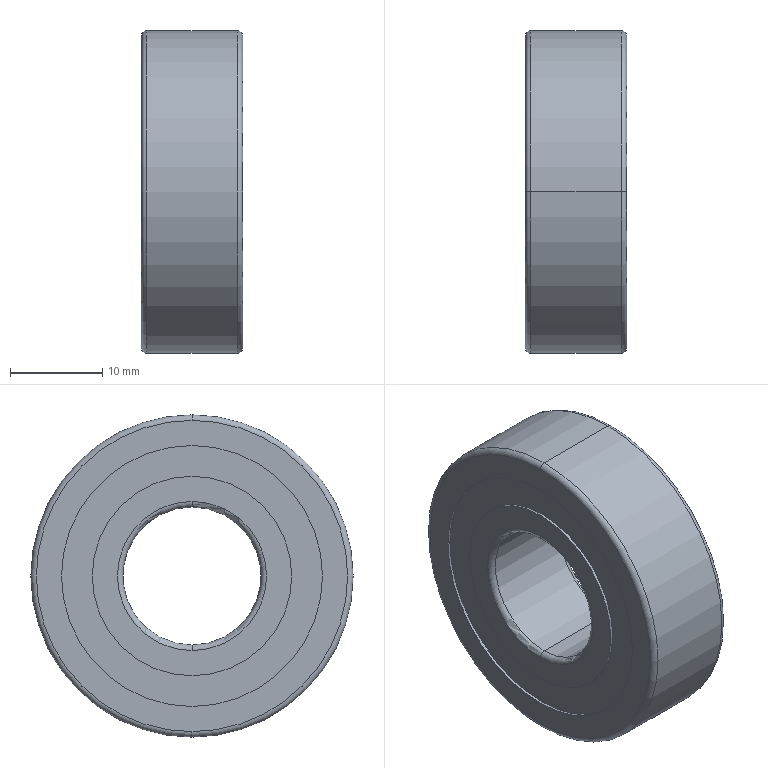Part | SolidWorks | features Revolution 3, CirPattern 1, RefAxis 1 | 17 solids | 88 faces | box 11 x 35 x 35 mm | volume 6620 mm3 | sphere 28 | cylinder 24 | torus 14 | cone 12 | plane 10 | commonest cylinder face diameters 21.667 x6 28.333 x6 20.467 x4 29.533 x4 15 x2 35 x2